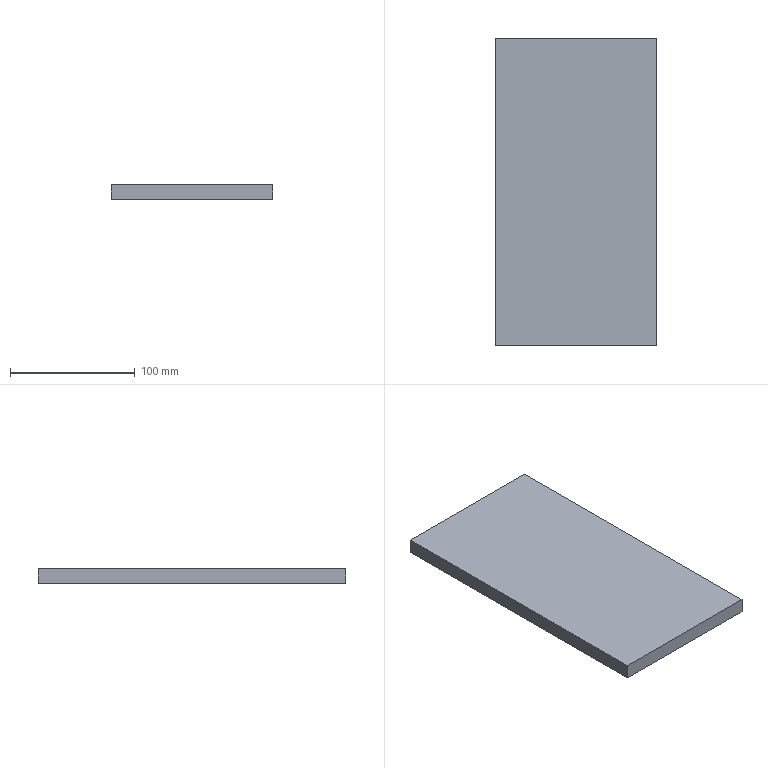Part | SolidWorks | features BaseBody 1 | 1 solid | 6 faces | box 130 x 247 x 12 mm | volume 385320 mm3 | plane 6
STEP:
#1=CARTESIAN_POINT('',(65.,-122.,0.));
#2=VERTEX_POINT('',#1);
#3=CARTESIAN_POINT('',(65.,-122.,12.));
#4=VERTEX_POINT('',#3);
#5=CARTESIAN_POINT('',(65.,-122.,12.));
#6=DIRECTION('',(0.,0.,1.));
#7=VECTOR('',#6,1000.);
#8=LINE('',#5,#7);
#9=EDGE_CURVE('',#2,#4,#8,.T.);
#10=ORIENTED_EDGE('',*,*,#9,.F.);
#11=CARTESIAN_POINT('',(65.,125.,0.));
#12=VERTEX_POINT('',#11);
#13=CARTESIAN_POINT('',(65.,125.,0.));
#14=DIRECTION('',(0.,1.,0.));
#15=VECTOR('',#14,1000.);
#16=LINE('',#13,#15);
#17=EDGE_CURVE('',#2,#12,#16,.T.);
#18=ORIENTED_EDGE('',*,*,#17,.T.);
#19=CARTESIAN_POINT('',(65.,125.,12.));
#20=VERTEX_POINT('',#19);
#21=CARTESIAN_POINT('',(65.,125.,12.));
#22=DIRECTION('',(0.,0.,-1.));
#23=VECTOR('',#22,1000.);
#24=LINE('',#21,#23);
#25=EDGE_CURVE('',#20,#12,#24,.T.);
#26=ORIENTED_EDGE('',*,*,#25,.F.);
#27=CARTESIAN_POINT('',(65.,125.,12.));
#28=DIRECTION('',(0.,1.,0.));
#29=VECTOR('',#28,1000.);
#30=LINE('',#27,#29);
#31=EDGE_CURVE('',#4,#20,#30,.T.);
#32=ORIENTED_EDGE('',*,*,#31,.F.);
#33=EDGE_LOOP('',(#10,#18,#26,#32));
#34=FACE_OUTER_BOUND('',#33,.T.);
#35=CARTESIAN_POINT('',(65.,125.,12.));
#36=DIRECTION('',(-1.,0.,0.));
#37=DIRECTION('',(0.,-1.,0.));
#38=AXIS2_PLACEMENT_3D('',#35,#36,#37);
#39=PLANE('',#38);
#40=ADVANCED_FACE('',(#34),#39,.F.);
#41=CARTESIAN_POINT('',(-65.,-122.,12.));
#42=VERTEX_POINT('',#41);
#43=CARTESIAN_POINT('',(-65.,-122.,0.));
#44=VERTEX_POINT('',#43);
#45=CARTESIAN_POINT('',(-65.,-122.,12.));
#46=DIRECTION('',(0.,0.,-1.));
#47=VECTOR('',#46,1000.);
#48=LINE('',#45,#47);
#49=EDGE_CURVE('',#42,#44,#48,.T.);
#50=ORIENTED_EDGE('',*,*,#49,.F.);
#51=CARTESIAN_POINT('',(-65.,125.,12.));
#52=VERTEX_POINT('',#51);
#53=CARTESIAN_POINT('',(-65.,125.,12.));
#54=DIRECTION('',(0.,-1.,0.));
#55=VECTOR('',#54,1000.);
#56=LINE('',#53,#55);
#57=EDGE_CURVE('',#52,#42,#56,.T.);
#58=ORIENTED_EDGE('',*,*,#57,.F.);
#59=CARTESIAN_POINT('',(-65.,125.,0.));
#60=VERTEX_POINT('',#59);
#61=CARTESIAN_POINT('',(-65.,125.,12.));
#62=DIRECTION('',(0.,0.,-1.));
#63=VECTOR('',#62,1000.);
#64=LINE('',#61,#63);
#65=EDGE_CURVE('',#52,#60,#64,.T.);
#66=ORIENTED_EDGE('',*,*,#65,.T.);
#67=CARTESIAN_POINT('',(-65.,125.,0.));
#68=DIRECTION('',(0.,-1.,0.));
#69=VECTOR('',#68,1000.);
#70=LINE('',#67,#69);
#71=EDGE_CURVE('',#60,#44,#70,.T.);
#72=ORIENTED_EDGE('',*,*,#71,.T.);
#73=EDGE_LOOP('',(#50,#58,#66,#72));
#74=FACE_OUTER_BOUND('',#73,.T.);
#75=CARTESIAN_POINT('',(-65.,125.,12.));
#76=DIRECTION('',(1.,0.,0.));
#77=DIRECTION('',(0.,1.,0.));
#78=AXIS2_PLACEMENT_3D('',#75,#76,#77);
#79=PLANE('',#78);
#80=ADVANCED_FACE('',(#74),#79,.F.);
#81=ORIENTED_EDGE('',*,*,#57,.T.);
#82=CARTESIAN_POINT('',(-85.,-122.,12.));
#83=DIRECTION('',(-1.,0.,0.));
#84=VECTOR('',#83,1000.);
#85=LINE('',#82,#84);
#86=EDGE_CURVE('',#4,#42,#85,.T.);
#87=ORIENTED_EDGE('',*,*,#86,.F.);
#88=ORIENTED_EDGE('',*,*,#31,.T.);
#89=CARTESIAN_POINT('',(-65.,125.,12.));
#90=DIRECTION('',(-1.,0.,0.));
#91=VECTOR('',#90,1000.);
#92=LINE('',#89,#91);
#93=EDGE_CURVE('',#20,#52,#92,.T.);
#94=ORIENTED_EDGE('',*,*,#93,.T.);
#95=EDGE_LOOP('',(#81,#87,#88,#94));
#96=FACE_OUTER_BOUND('',#95,.T.);
#97=CARTESIAN_POINT('',(0.,0.,12.));
#98=DIRECTION('',(0.,0.,1.));
#99=DIRECTION('',(1.,0.,0.));
#100=AXIS2_PLACEMENT_3D('',#97,#98,#99);
#101=PLANE('',#100);
#102=ADVANCED_FACE('',(#96),#101,.T.);
#103=CARTESIAN_POINT('',(0.,-122.,0.));
#104=DIRECTION('',(1.,0.,0.));
#105=VECTOR('',#104,1000.);
#106=LINE('',#103,#105);
#107=EDGE_CURVE('',#44,#2,#106,.T.);
#108=ORIENTED_EDGE('',*,*,#107,.F.);
#109=ORIENTED_EDGE('',*,*,#71,.F.);
#110=CARTESIAN_POINT('',(-65.,125.,0.));
#111=DIRECTION('',(-1.,0.,0.));
#112=VECTOR('',#111,1000.);
#113=LINE('',#110,#112);
#114=EDGE_CURVE('',#12,#60,#113,.T.);
#115=ORIENTED_EDGE('',*,*,#114,.F.);
#116=ORIENTED_EDGE('',*,*,#17,.F.);
#117=EDGE_LOOP('',(#108,#109,#115,#116));
#118=FACE_OUTER_BOUND('',#117,.T.);
#119=CARTESIAN_POINT('',(0.,0.,0.));
#120=DIRECTION('',(0.,0.,1.));
#121=DIRECTION('',(1.,0.,0.));
#122=AXIS2_PLACEMENT_3D('',#119,#120,#121);
#123=PLANE('',#122);
#124=ADVANCED_FACE('',(#118),#123,.F.);
#125=ORIENTED_EDGE('',*,*,#114,.T.);
#126=ORIENTED_EDGE('',*,*,#65,.F.);
#127=ORIENTED_EDGE('',*,*,#93,.F.);
#128=ORIENTED_EDGE('',*,*,#25,.T.);
#129=EDGE_LOOP('',(#125,#126,#127,#128));
#130=FACE_OUTER_BOUND('',#129,.T.);
#131=CARTESIAN_POINT('',(-65.,125.,12.));
#132=DIRECTION('',(0.,-1.,0.));
#133=DIRECTION('',(1.,0.,0.));
#134=AXIS2_PLACEMENT_3D('',#131,#132,#133);
#135=PLANE('',#134);
#136=ADVANCED_FACE('',(#130),#135,.F.);
#137=ORIENTED_EDGE('',*,*,#9,.T.);
#138=ORIENTED_EDGE('',*,*,#86,.T.);
#139=ORIENTED_EDGE('',*,*,#49,.T.);
#140=ORIENTED_EDGE('',*,*,#107,.T.);
#141=EDGE_LOOP('',(#137,#138,#139,#140));
#142=FACE_OUTER_BOUND('',#141,.T.);
#143=CARTESIAN_POINT('',(0.,-122.,-763.));
#144=DIRECTION('',(0.,-1.,0.));
#145=DIRECTION('',(1.,0.,0.));
#146=AXIS2_PLACEMENT_3D('',#143,#144,#145);
#147=PLANE('',#146);
#148=ADVANCED_FACE('',(#142),#147,.T.);
#149=CLOSED_SHELL('',(#40,#80,#102,#124,#136,#148));
#150=MANIFOLD_SOLID_BREP('',#149);
#151=CARTESIAN_POINT('',(0.,0.,0.));
#152=DIRECTION('',(0.,0.,1.));
#153=DIRECTION('',(1.,0.,0.));
#154=AXIS2_PLACEMENT_3D('',#151,#152,#153);
#155=(LENGTH_UNIT()NAMED_UNIT(*)SI_UNIT(.MILLI.,.METRE.));
#156=UNCERTAINTY_MEASURE_WITH_UNIT(LENGTH_MEASURE(0.00001),#155,'','');
#157=(NAMED_UNIT(*)PLANE_ANGLE_UNIT()SI_UNIT($,.RADIAN.));
#158=(NAMED_UNIT(*)SI_UNIT($,.STERADIAN.)SOLID_ANGLE_UNIT());
#159=(GEOMETRIC_REPRESENTATION_CONTEXT(3)GLOBAL_UNCERTAINTY_ASSIGNED_CONTEXT((#156))GLOBAL_UNIT_ASSIGNED_CONTEXT((#155,#157,#158))REPRESENTATION_CONTEXT('',''));
#160=ADVANCED_BREP_SHAPE_REPRESENTATION('',(#150,#154),#159);